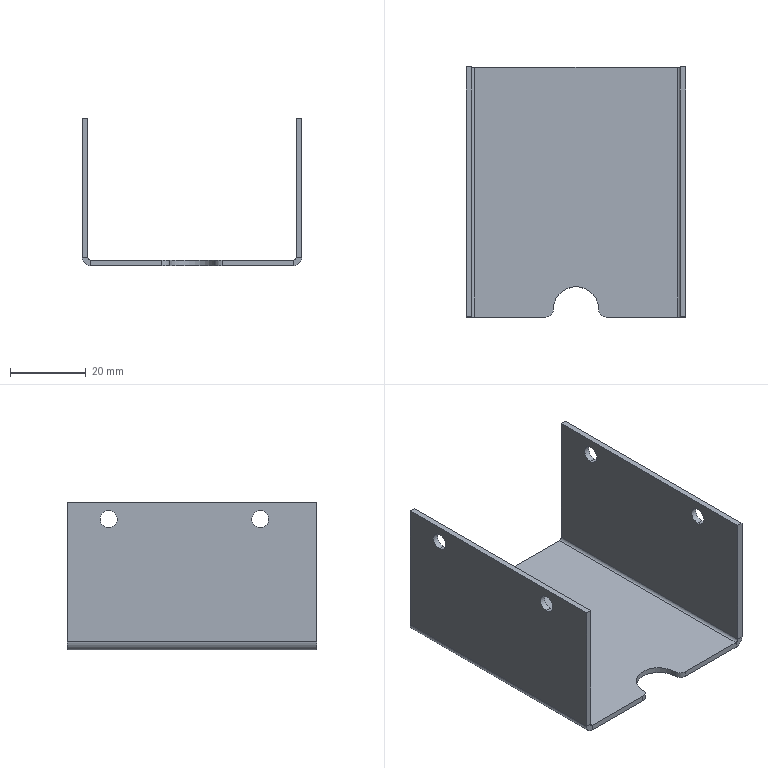Part | STEP file | PN_0075 Mount electronic clip s longitudinal manipulator fixture | 1 solid | 34 faces | box 58 x 66 x 39 mm | volume 12822 mm3 | plane 19 | cylinder 15 | commonest cylinder face diameters 4.5 x8 1.473 x2 4 x2 4.473 x2 12 x1